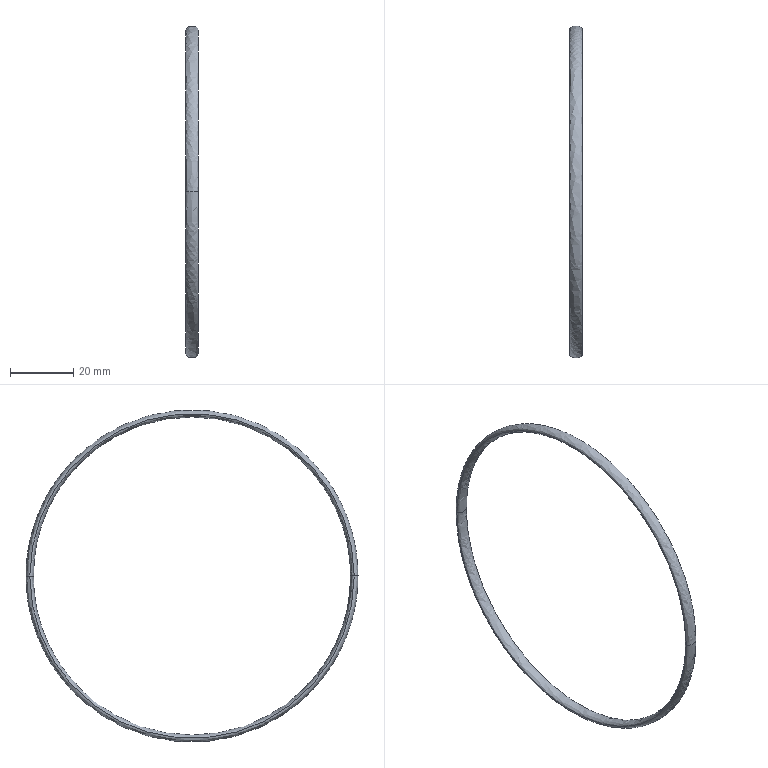Part | SolidWorks | features Revolution 2 | 1 solid | 4 faces | box 4 x 105 x 105 mm | volume 2430 mm3 | spline 4
STEP:
#1=CARTESIAN_POINT('',(4.,51.3,0.));
#2=VERTEX_POINT('',#1);
#3=CARTESIAN_POINT('',(4.,-51.3,0.));
#4=VERTEX_POINT('',#3);
#5=CARTESIAN_POINT('',(4.,0.,0.));
#6=DIRECTION('',(-1.,0.,0.));
#7=DIRECTION('',(0.,1.,0.));
#8=AXIS2_PLACEMENT_3D('',#5,#6,#7);
#9=CIRCLE('',#8,51.3);
#10=EDGE_CURVE('',#2,#4,#9,.T.);
#11=ORIENTED_EDGE('',*,*,#10,.T.);
#12=CARTESIAN_POINT('',(0.,-51.3,0.));
#13=VERTEX_POINT('',#12);
#14=CARTESIAN_POINT('',(4.,-51.3,0.));
#15=CARTESIAN_POINT('',(4.,-53.7,0.));
#16=CARTESIAN_POINT('',(0.,-53.7,0.));
#17=CARTESIAN_POINT('',(0.,-51.3,0.));
#18=(BOUNDED_CURVE()B_SPLINE_CURVE(3,(#14,#15,#16,#17),.UNSPECIFIED.,.F.,.F.)B_SPLINE_CURVE_WITH_KNOTS((4,4),(0.,3.142),.UNSPECIFIED.)CURVE()GEOMETRIC_REPRESENTATION_ITEM()RATIONAL_B_SPLINE_CURVE((1.,0.3333,0.3333,1.))REPRESENTATION_ITEM(''));
#19=EDGE_CURVE('',#4,#13,#18,.T.);
#20=ORIENTED_EDGE('',*,*,#19,.T.);
#21=CARTESIAN_POINT('',(0.,51.3,0.));
#22=VERTEX_POINT('',#21);
#23=CARTESIAN_POINT('',(0.,0.,0.));
#24=DIRECTION('',(-1.,0.,0.));
#25=DIRECTION('',(0.,1.,0.));
#26=AXIS2_PLACEMENT_3D('',#23,#24,#25);
#27=CIRCLE('',#26,51.3);
#28=EDGE_CURVE('',#22,#13,#27,.T.);
#29=ORIENTED_EDGE('',*,*,#28,.F.);
#30=CARTESIAN_POINT('',(4.,51.3,0.));
#31=CARTESIAN_POINT('',(4.,53.7,0.));
#32=CARTESIAN_POINT('',(0.,53.7,0.));
#33=CARTESIAN_POINT('',(0.,51.3,0.));
#34=(BOUNDED_CURVE()B_SPLINE_CURVE(3,(#30,#31,#32,#33),.UNSPECIFIED.,.F.,.T.)B_SPLINE_CURVE_WITH_KNOTS((4,4),(0.,3.142),.UNSPECIFIED.)CURVE()GEOMETRIC_REPRESENTATION_ITEM()RATIONAL_B_SPLINE_CURVE((1.,0.3333,0.3333,1.))REPRESENTATION_ITEM(''));
#35=EDGE_CURVE('',#2,#22,#34,.T.);
#36=ORIENTED_EDGE('',*,*,#35,.F.);
#37=EDGE_LOOP('',(#11,#20,#29,#36));
#38=FACE_OUTER_BOUND('',#37,.T.);
#39=CARTESIAN_POINT('',(4.,51.3,0.));
#40=CARTESIAN_POINT('',(4.,51.3,-102.6));
#41=CARTESIAN_POINT('',(4.,-51.3,-102.6));
#42=CARTESIAN_POINT('',(4.,-51.3,0.));
#43=CARTESIAN_POINT('',(4.,53.7,0.));
#44=CARTESIAN_POINT('',(4.,53.7,-107.4));
#45=CARTESIAN_POINT('',(4.,-53.7,-107.4));
#46=CARTESIAN_POINT('',(4.,-53.7,0.));
#47=CARTESIAN_POINT('',(0.,53.7,0.));
#48=CARTESIAN_POINT('',(0.,53.7,-107.4));
#49=CARTESIAN_POINT('',(0.,-53.7,-107.4));
#50=CARTESIAN_POINT('',(0.,-53.7,0.));
#51=CARTESIAN_POINT('',(0.,51.3,0.));
#52=CARTESIAN_POINT('',(0.,51.3,-102.6));
#53=CARTESIAN_POINT('',(0.,-51.3,-102.6));
#54=CARTESIAN_POINT('',(0.,-51.3,0.));
#55=(BOUNDED_SURFACE()B_SPLINE_SURFACE(3,3,((#39,#40,#41,#42),(#43,#44,#45,#46),(#47,#48,#49,#50),(#51,#52,#53,#54)),.UNSPECIFIED.,.F.,.F.,.T.)B_SPLINE_SURFACE_WITH_KNOTS((4,4),(4,4),(0.,1.),(0.,1.),.UNSPECIFIED.)GEOMETRIC_REPRESENTATION_ITEM()RATIONAL_B_SPLINE_SURFACE(((1.,0.3333,0.3333,1.),(0.3333,0.1111,0.1111,0.3333),(0.3333,0.1111,0.1111,0.3333),(1.,0.3333,0.3333,1.)))REPRESENTATION_ITEM('')SURFACE());
#56=ADVANCED_FACE('',(#38),#55,.F.);
#57=ORIENTED_EDGE('',*,*,#28,.T.);
#58=CARTESIAN_POINT('',(0.,-51.3,0.));
#59=CARTESIAN_POINT('',(0.,-48.9,0.));
#60=CARTESIAN_POINT('',(4.,-48.9,0.));
#61=CARTESIAN_POINT('',(4.,-51.3,0.));
#62=(BOUNDED_CURVE()B_SPLINE_CURVE(3,(#58,#59,#60,#61),.UNSPECIFIED.,.F.,.F.)B_SPLINE_CURVE_WITH_KNOTS((4,4),(3.142,6.283),.UNSPECIFIED.)CURVE()GEOMETRIC_REPRESENTATION_ITEM()RATIONAL_B_SPLINE_CURVE((1.,0.3333,0.3333,1.))REPRESENTATION_ITEM(''));
#63=EDGE_CURVE('',#13,#4,#62,.T.);
#64=ORIENTED_EDGE('',*,*,#63,.T.);
#65=ORIENTED_EDGE('',*,*,#10,.F.);
#66=CARTESIAN_POINT('',(0.,51.3,0.));
#67=CARTESIAN_POINT('',(0.,48.9,0.));
#68=CARTESIAN_POINT('',(4.,48.9,0.));
#69=CARTESIAN_POINT('',(4.,51.3,0.));
#70=(BOUNDED_CURVE()B_SPLINE_CURVE(3,(#66,#67,#68,#69),.UNSPECIFIED.,.F.,.T.)B_SPLINE_CURVE_WITH_KNOTS((4,4),(3.142,6.283),.UNSPECIFIED.)CURVE()GEOMETRIC_REPRESENTATION_ITEM()RATIONAL_B_SPLINE_CURVE((1.,0.3333,0.3333,1.))REPRESENTATION_ITEM(''));
#71=EDGE_CURVE('',#22,#2,#70,.T.);
#72=ORIENTED_EDGE('',*,*,#71,.F.);
#73=EDGE_LOOP('',(#57,#64,#65,#72));
#74=FACE_OUTER_BOUND('',#73,.T.);
#75=CARTESIAN_POINT('',(0.,51.3,0.));
#76=CARTESIAN_POINT('',(0.,51.3,-102.6));
#77=CARTESIAN_POINT('',(0.,-51.3,-102.6));
#78=CARTESIAN_POINT('',(0.,-51.3,0.));
#79=CARTESIAN_POINT('',(0.,48.9,0.));
#80=CARTESIAN_POINT('',(0.,48.9,-97.8));
#81=CARTESIAN_POINT('',(0.,-48.9,-97.8));
#82=CARTESIAN_POINT('',(0.,-48.9,0.));
#83=CARTESIAN_POINT('',(4.,48.9,0.));
#84=CARTESIAN_POINT('',(4.,48.9,-97.8));
#85=CARTESIAN_POINT('',(4.,-48.9,-97.8));
#86=CARTESIAN_POINT('',(4.,-48.9,0.));
#87=CARTESIAN_POINT('',(4.,51.3,0.));
#88=CARTESIAN_POINT('',(4.,51.3,-102.6));
#89=CARTESIAN_POINT('',(4.,-51.3,-102.6));
#90=CARTESIAN_POINT('',(4.,-51.3,0.));
#91=(BOUNDED_SURFACE()B_SPLINE_SURFACE(3,3,((#75,#76,#77,#78),(#79,#80,#81,#82),(#83,#84,#85,#86),(#87,#88,#89,#90)),.UNSPECIFIED.,.F.,.F.,.T.)B_SPLINE_SURFACE_WITH_KNOTS((4,4),(4,4),(0.,1.),(0.,1.),.UNSPECIFIED.)GEOMETRIC_REPRESENTATION_ITEM()RATIONAL_B_SPLINE_SURFACE(((1.,0.3333,0.3333,1.),(0.3333,0.1111,0.1111,0.3333),(0.3333,0.1111,0.1111,0.3333),(1.,0.3333,0.3333,1.)))REPRESENTATION_ITEM('')SURFACE());
#92=ADVANCED_FACE('',(#74),#91,.F.);
#93=ORIENTED_EDGE('',*,*,#63,.F.);
#94=CARTESIAN_POINT('',(0.,0.,0.));
#95=DIRECTION('',(-1.,0.,0.));
#96=DIRECTION('',(0.,1.,0.));
#97=AXIS2_PLACEMENT_3D('',#94,#95,#96);
#98=CIRCLE('',#97,51.3);
#99=EDGE_CURVE('',#13,#22,#98,.T.);
#100=ORIENTED_EDGE('',*,*,#99,.T.);
#101=ORIENTED_EDGE('',*,*,#71,.T.);
#102=CARTESIAN_POINT('',(4.,0.,0.));
#103=DIRECTION('',(-1.,0.,0.));
#104=DIRECTION('',(0.,1.,0.));
#105=AXIS2_PLACEMENT_3D('',#102,#103,#104);
#106=CIRCLE('',#105,51.3);
#107=EDGE_CURVE('',#4,#2,#106,.T.);
#108=ORIENTED_EDGE('',*,*,#107,.F.);
#109=EDGE_LOOP('',(#93,#100,#101,#108));
#110=FACE_OUTER_BOUND('',#109,.T.);
#111=CARTESIAN_POINT('',(0.,-51.3,0.));
#112=CARTESIAN_POINT('',(0.,-51.3,102.6));
#113=CARTESIAN_POINT('',(0.,51.3,102.6));
#114=CARTESIAN_POINT('',(0.,51.3,0.));
#115=CARTESIAN_POINT('',(0.,-48.9,0.));
#116=CARTESIAN_POINT('',(0.,-48.9,97.8));
#117=CARTESIAN_POINT('',(0.,48.9,97.8));
#118=CARTESIAN_POINT('',(0.,48.9,0.));
#119=CARTESIAN_POINT('',(4.,-48.9,0.));
#120=CARTESIAN_POINT('',(4.,-48.9,97.8));
#121=CARTESIAN_POINT('',(4.,48.9,97.8));
#122=CARTESIAN_POINT('',(4.,48.9,0.));
#123=CARTESIAN_POINT('',(4.,-51.3,0.));
#124=CARTESIAN_POINT('',(4.,-51.3,102.6));
#125=CARTESIAN_POINT('',(4.,51.3,102.6));
#126=CARTESIAN_POINT('',(4.,51.3,0.));
#127=(BOUNDED_SURFACE()B_SPLINE_SURFACE(3,3,((#111,#112,#113,#114),(#115,#116,#117,#118),(#119,#120,#121,#122),(#123,#124,#125,#126)),.UNSPECIFIED.,.F.,.F.,.T.)B_SPLINE_SURFACE_WITH_KNOTS((4,4),(4,4),(0.,1.),(0.,1.),.UNSPECIFIED.)GEOMETRIC_REPRESENTATION_ITEM()RATIONAL_B_SPLINE_SURFACE(((1.,0.3333,0.3333,1.),(0.3333,0.1111,0.1111,0.3333),(0.3333,0.1111,0.1111,0.3333),(1.,0.3333,0.3333,1.)))REPRESENTATION_ITEM('')SURFACE());
#128=ADVANCED_FACE('',(#110),#127,.F.);
#129=ORIENTED_EDGE('',*,*,#19,.F.);
#130=ORIENTED_EDGE('',*,*,#107,.T.);
#131=ORIENTED_EDGE('',*,*,#35,.T.);
#132=ORIENTED_EDGE('',*,*,#99,.F.);
#133=EDGE_LOOP('',(#129,#130,#131,#132));
#134=FACE_OUTER_BOUND('',#133,.T.);
#135=CARTESIAN_POINT('',(4.,-51.3,0.));
#136=CARTESIAN_POINT('',(4.,-51.3,102.6));
#137=CARTESIAN_POINT('',(4.,51.3,102.6));
#138=CARTESIAN_POINT('',(4.,51.3,0.));
#139=CARTESIAN_POINT('',(4.,-53.7,0.));
#140=CARTESIAN_POINT('',(4.,-53.7,107.4));
#141=CARTESIAN_POINT('',(4.,53.7,107.4));
#142=CARTESIAN_POINT('',(4.,53.7,0.));
#143=CARTESIAN_POINT('',(0.,-53.7,0.));
#144=CARTESIAN_POINT('',(0.,-53.7,107.4));
#145=CARTESIAN_POINT('',(0.,53.7,107.4));
#146=CARTESIAN_POINT('',(0.,53.7,0.));
#147=CARTESIAN_POINT('',(0.,-51.3,0.));
#148=CARTESIAN_POINT('',(0.,-51.3,102.6));
#149=CARTESIAN_POINT('',(0.,51.3,102.6));
#150=CARTESIAN_POINT('',(0.,51.3,0.));
#151=(BOUNDED_SURFACE()B_SPLINE_SURFACE(3,3,((#135,#136,#137,#138),(#139,#140,#141,#142),(#143,#144,#145,#146),(#147,#148,#149,#150)),.UNSPECIFIED.,.F.,.F.,.T.)B_SPLINE_SURFACE_WITH_KNOTS((4,4),(4,4),(0.,1.),(0.,1.),.UNSPECIFIED.)GEOMETRIC_REPRESENTATION_ITEM()RATIONAL_B_SPLINE_SURFACE(((1.,0.3333,0.3333,1.),(0.3333,0.1111,0.1111,0.3333),(0.3333,0.1111,0.1111,0.3333),(1.,0.3333,0.3333,1.)))REPRESENTATION_ITEM('')SURFACE());
#152=ADVANCED_FACE('',(#134),#151,.F.);
#153=CLOSED_SHELL('',(#56,#92,#128,#152));
#154=MANIFOLD_SOLID_BREP('',#153);
#155=CARTESIAN_POINT('',(0.,0.,0.));
#156=DIRECTION('',(0.,0.,1.));
#157=DIRECTION('',(1.,0.,0.));
#158=AXIS2_PLACEMENT_3D('',#155,#156,#157);
#159=(LENGTH_UNIT()NAMED_UNIT(*)SI_UNIT(.MILLI.,.METRE.));
#160=UNCERTAINTY_MEASURE_WITH_UNIT(LENGTH_MEASURE(0.00001),#159,'','');
#161=(NAMED_UNIT(*)PLANE_ANGLE_UNIT()SI_UNIT($,.RADIAN.));
#162=(NAMED_UNIT(*)SI_UNIT($,.STERADIAN.)SOLID_ANGLE_UNIT());
#163=(GEOMETRIC_REPRESENTATION_CONTEXT(3)GLOBAL_UNCERTAINTY_ASSIGNED_CONTEXT((#160))GLOBAL_UNIT_ASSIGNED_CONTEXT((#159,#161,#162))REPRESENTATION_CONTEXT('',''));
#164=ADVANCED_BREP_SHAPE_REPRESENTATION('',(#154,#158),#163);